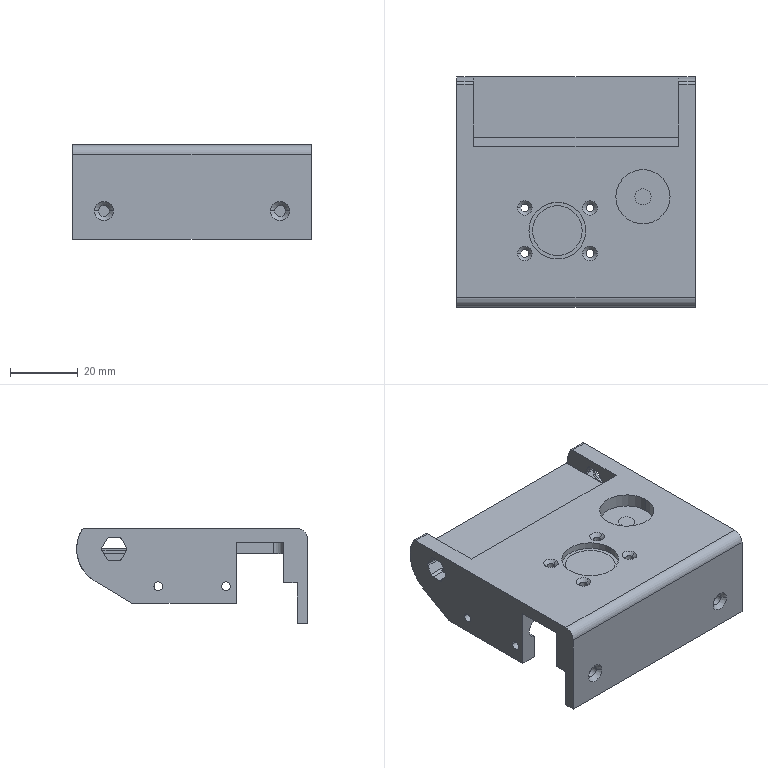NC program | NX | posted with a generic post | part box 70.5 x 68.1 x 28 mm
Whole program:
N10 G17 G21 G94 G90
(DRILLING_COPY , TOOL : D6A45)
N12 T07 M6
N14 G54
N16 G17 G0 G90 X-29.5 Y-11.8 B0. C0. S3500 M3
N18 G43 Z98.1 H7
N20 G94 G81 G98 Z65.95 F250. R71.1
N22 X29.5
N24 G80
N26 G0 X29.5 Y-11.8 Z98.1
N28 M5
(DRILLING_COPY_COPY_COPY_COPY , TOOL : 6.0ZT)
N30 T16 M6
N32 G54
N34 G17 G0 G90 X29.5 Y-11.8 B0. C0. S2500 M3
N36 G43 Z98.1 H16
N38 G94 G83 G98 Z17.697 F120. Q2. R71.1
N40 X-29.5 Z41.797
N42 G80
N44 G0 X-29.5 Y-11.8 Z98.1
N46 M5
N48 M2